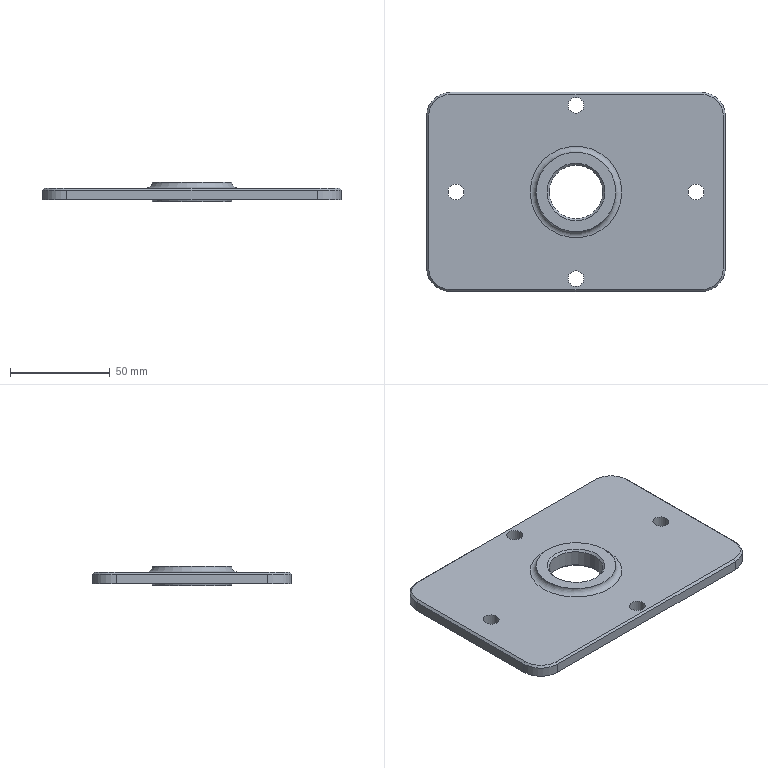Part | NX | features DATUM_CSYS 2, BLEND 1, BREP 1, CHAMFER 1, CPROJ 1, EXTRUDE 1, SKETCH 1 | 1 solid | 38 faces | box 150 x 100 x 10 mm | volume 75362 mm3 | plane 13 | cylinder 13 | cone 6 | torus 6 | commonest cylinder face diameters 4 x4 8 x4 24 x4 27 x1
STEP:
#1=CARTESIAN_POINT('',(15.75,378.,376.084));
#2=VERTEX_POINT('',#1);
#3=CARTESIAN_POINT('',(19.75,378.,376.084));
#4=DIRECTION('',(0.,0.,-1.));
#5=DIRECTION('',(-1.,0.,0.));
#6=AXIS2_PLACEMENT_3D('',#3,#4,#5);
#7=CIRCLE('',#6,4.);
#8=EDGE_CURVE('',#2,#2,#7,.T.);
#9=ORIENTED_EDGE('',*,*,#8,.F.);
#10=EDGE_LOOP('',(#9));
#11=FACE_BOUND('',#10,.T.);
#12=CARTESIAN_POINT('',(136.25,378.,376.084));
#13=VERTEX_POINT('',#12);
#14=CARTESIAN_POINT('',(140.25,378.,376.084));
#15=DIRECTION('',(0.,0.,-1.));
#16=DIRECTION('',(-1.,0.,0.));
#17=AXIS2_PLACEMENT_3D('',#14,#15,#16);
#18=CIRCLE('',#17,4.);
#19=EDGE_CURVE('',#13,#13,#18,.T.);
#20=ORIENTED_EDGE('',*,*,#19,.F.);
#21=EDGE_LOOP('',(#20));
#22=FACE_BOUND('',#21,.T.);
#23=CARTESIAN_POINT('',(126.,340.5,376.084));
#24=VERTEX_POINT('',#23);
#25=CARTESIAN_POINT('',(130.,344.5,376.084));
#26=VERTEX_POINT('',#25);
#27=CARTESIAN_POINT('',(126.,344.5,376.084));
#28=DIRECTION('',(0.,0.,1.));
#29=DIRECTION('',(1.,0.,0.));
#30=AXIS2_PLACEMENT_3D('',#27,#28,#29);
#31=CIRCLE('',#30,4.);
#32=EDGE_CURVE('',#24,#26,#31,.T.);
#33=ORIENTED_EDGE('',*,*,#32,.T.);
#34=CARTESIAN_POINT('',(130.,411.5,376.084));
#35=VERTEX_POINT('',#34);
#36=CARTESIAN_POINT('',(130.,344.5,376.084));
#37=DIRECTION('',(0.,-1.,0.));
#38=VECTOR('',#37,1000.);
#39=LINE('',#36,#38);
#40=EDGE_CURVE('',#26,#35,#39,.F.);
#41=ORIENTED_EDGE('',*,*,#40,.T.);
#42=CARTESIAN_POINT('',(126.,415.5,376.084));
#43=VERTEX_POINT('',#42);
#44=CARTESIAN_POINT('',(126.,411.5,376.084));
#45=DIRECTION('',(0.,0.,1.));
#46=DIRECTION('',(1.,0.,0.));
#47=AXIS2_PLACEMENT_3D('',#44,#45,#46);
#48=CIRCLE('',#47,4.);
#49=EDGE_CURVE('',#35,#43,#48,.T.);
#50=ORIENTED_EDGE('',*,*,#49,.T.);
#51=CARTESIAN_POINT('',(34.,415.5,376.084));
#52=VERTEX_POINT('',#51);
#53=CARTESIAN_POINT('',(126.,415.5,376.084));
#54=DIRECTION('',(1.,0.,0.));
#55=VECTOR('',#54,1000.);
#56=LINE('',#53,#55);
#57=EDGE_CURVE('',#43,#52,#56,.F.);
#58=ORIENTED_EDGE('',*,*,#57,.T.);
#59=CARTESIAN_POINT('',(30.,411.5,376.084));
#60=VERTEX_POINT('',#59);
#61=CARTESIAN_POINT('',(34.,411.5,376.084));
#62=DIRECTION('',(0.,0.,1.));
#63=DIRECTION('',(1.,0.,0.));
#64=AXIS2_PLACEMENT_3D('',#61,#62,#63);
#65=CIRCLE('',#64,4.);
#66=EDGE_CURVE('',#52,#60,#65,.T.);
#67=ORIENTED_EDGE('',*,*,#66,.T.);
#68=CARTESIAN_POINT('',(30.,344.5,376.084));
#69=VERTEX_POINT('',#68);
#70=CARTESIAN_POINT('',(30.,411.5,376.084));
#71=DIRECTION('',(0.,1.,0.));
#72=VECTOR('',#71,1000.);
#73=LINE('',#70,#72);
#74=EDGE_CURVE('',#60,#69,#73,.F.);
#75=ORIENTED_EDGE('',*,*,#74,.T.);
#76=CARTESIAN_POINT('',(34.,340.5,376.084));
#77=VERTEX_POINT('',#76);
#78=CARTESIAN_POINT('',(34.,344.5,376.084));
#79=DIRECTION('',(0.,0.,1.));
#80=DIRECTION('',(1.,0.,0.));
#81=AXIS2_PLACEMENT_3D('',#78,#79,#80);
#82=CIRCLE('',#81,4.);
#83=EDGE_CURVE('',#69,#77,#82,.T.);
#84=ORIENTED_EDGE('',*,*,#83,.T.);
#85=CARTESIAN_POINT('',(34.,340.5,376.084));
#86=DIRECTION('',(-1.,0.,0.));
#87=VECTOR('',#86,1000.);
#88=LINE('',#85,#87);
#89=EDGE_CURVE('',#77,#24,#88,.F.);
#90=ORIENTED_EDGE('',*,*,#89,.T.);
#91=EDGE_LOOP('',(#33,#41,#50,#58,#67,#75,#84,#90));
#92=FACE_BOUND('',#91,.T.);
#93=CARTESIAN_POINT('',(155.,416.,376.084));
#94=VERTEX_POINT('',#93);
#95=CARTESIAN_POINT('',(155.,340.,376.084));
#96=VERTEX_POINT('',#95);
#97=CARTESIAN_POINT('',(155.,516.,376.084));
#98=DIRECTION('',(0.,1.,0.));
#99=VECTOR('',#98,1000.);
#100=LINE('',#97,#99);
#101=EDGE_CURVE('',#94,#96,#100,.F.);
#102=ORIENTED_EDGE('',*,*,#101,.T.);
#103=CARTESIAN_POINT('',(143.,328.,376.084));
#104=VERTEX_POINT('',#103);
#105=CARTESIAN_POINT('',(143.,340.,376.084));
#106=DIRECTION('',(0.,0.,1.));
#107=DIRECTION('',(1.,0.,0.));
#108=AXIS2_PLACEMENT_3D('',#105,#106,#107);
#109=CIRCLE('',#108,12.);
#110=EDGE_CURVE('',#96,#104,#109,.F.);
#111=ORIENTED_EDGE('',*,*,#110,.T.);
#112=CARTESIAN_POINT('',(17.,328.,376.084));
#113=VERTEX_POINT('',#112);
#114=CARTESIAN_POINT('',(160.,328.,376.084));
#115=DIRECTION('',(1.,0.,0.));
#116=VECTOR('',#115,1000.);
#117=LINE('',#114,#116);
#118=EDGE_CURVE('',#104,#113,#117,.F.);
#119=ORIENTED_EDGE('',*,*,#118,.T.);
#120=CARTESIAN_POINT('',(5.,340.,376.084));
#121=VERTEX_POINT('',#120);
#122=CARTESIAN_POINT('',(17.,340.,376.084));
#123=DIRECTION('',(0.,0.,1.));
#124=DIRECTION('',(1.,0.,0.));
#125=AXIS2_PLACEMENT_3D('',#122,#123,#124);
#126=CIRCLE('',#125,12.);
#127=EDGE_CURVE('',#113,#121,#126,.F.);
#128=ORIENTED_EDGE('',*,*,#127,.T.);
#129=CARTESIAN_POINT('',(5.,416.,376.084));
#130=VERTEX_POINT('',#129);
#131=CARTESIAN_POINT('',(5.,516.,376.084));
#132=DIRECTION('',(0.,-1.,0.));
#133=VECTOR('',#132,1000.);
#134=LINE('',#131,#133);
#135=EDGE_CURVE('',#121,#130,#134,.F.);
#136=ORIENTED_EDGE('',*,*,#135,.T.);
#137=CARTESIAN_POINT('',(17.,428.,376.084));
#138=VERTEX_POINT('',#137);
#139=CARTESIAN_POINT('',(17.,416.,376.084));
#140=DIRECTION('',(0.,0.,1.));
#141=DIRECTION('',(1.,0.,0.));
#142=AXIS2_PLACEMENT_3D('',#139,#140,#141);
#143=CIRCLE('',#142,12.);
#144=EDGE_CURVE('',#138,#130,#143,.T.);
#145=ORIENTED_EDGE('',*,*,#144,.F.);
#146=CARTESIAN_POINT('',(143.,428.,376.084));
#147=VERTEX_POINT('',#146);
#148=CARTESIAN_POINT('',(160.,428.,376.084));
#149=DIRECTION('',(-1.,0.,0.));
#150=VECTOR('',#149,1000.);
#151=LINE('',#148,#150);
#152=EDGE_CURVE('',#138,#147,#151,.F.);
#153=ORIENTED_EDGE('',*,*,#152,.T.);
#154=CARTESIAN_POINT('',(143.,416.,376.084));
#155=DIRECTION('',(0.,0.,1.));
#156=DIRECTION('',(1.,0.,0.));
#157=AXIS2_PLACEMENT_3D('',#154,#155,#156);
#158=CIRCLE('',#157,12.);
#159=EDGE_CURVE('',#147,#94,#158,.F.);
#160=ORIENTED_EDGE('',*,*,#159,.T.);
#161=EDGE_LOOP('',(#102,#111,#119,#128,#136,#145,#153,#160));
#162=FACE_BOUND('',#161,.T.);
#163=CARTESIAN_POINT('',(76.,334.5,376.084));
#164=VERTEX_POINT('',#163);
#165=CARTESIAN_POINT('',(80.,334.5,376.084));
#166=DIRECTION('',(0.,0.,-1.));
#167=DIRECTION('',(-1.,0.,0.));
#168=AXIS2_PLACEMENT_3D('',#165,#166,#167);
#169=CIRCLE('',#168,4.);
#170=EDGE_CURVE('',#164,#164,#169,.T.);
#171=ORIENTED_EDGE('',*,*,#170,.F.);
#172=EDGE_LOOP('',(#171));
#173=FACE_BOUND('',#172,.T.);
#174=CARTESIAN_POINT('',(76.,421.5,376.084));
#175=VERTEX_POINT('',#174);
#176=CARTESIAN_POINT('',(80.,421.5,376.084));
#177=DIRECTION('',(0.,0.,-1.));
#178=DIRECTION('',(-1.,0.,0.));
#179=AXIS2_PLACEMENT_3D('',#176,#177,#178);
#180=CIRCLE('',#179,4.);
#181=EDGE_CURVE('',#175,#175,#180,.F.);
#182=ORIENTED_EDGE('',*,*,#181,.T.);
#183=EDGE_LOOP('',(#182));
#184=FACE_BOUND('',#183,.T.);
#185=CARTESIAN_POINT('',(80.,378.,376.084));
#186=DIRECTION('',(0.,0.,-1.));
#187=DIRECTION('',(-1.,0.,0.));
#188=AXIS2_PLACEMENT_3D('',#185,#186,#187);
#189=PLANE('',#188);
#190=ADVANCED_FACE('',(#11,#22,#92,#162,#173,#184),#189,.T.);
#191=CARTESIAN_POINT('',(76.,334.5,382.084));
#192=VERTEX_POINT('',#191);
#193=CARTESIAN_POINT('',(80.,334.5,382.084));
#194=DIRECTION('',(0.,0.,-1.));
#195=DIRECTION('',(-1.,0.,0.));
#196=AXIS2_PLACEMENT_3D('',#193,#194,#195);
#197=CIRCLE('',#196,4.);
#198=EDGE_CURVE('',#192,#192,#197,.F.);
#199=ORIENTED_EDGE('',*,*,#198,.T.);
#200=EDGE_LOOP('',(#199));
#201=FACE_BOUND('',#200,.T.);
#202=ORIENTED_EDGE('',*,*,#170,.T.);
#203=EDGE_LOOP('',(#202));
#204=FACE_BOUND('',#203,.T.);
#205=CARTESIAN_POINT('',(80.,334.5,402.084));
#206=DIRECTION('',(0.,0.,-1.));
#207=DIRECTION('',(-1.,0.,0.));
#208=AXIS2_PLACEMENT_3D('',#205,#206,#207);
#209=CYLINDRICAL_SURFACE('',#208,4.);
#210=ADVANCED_FACE('',(#201,#204),#209,.F.);
#211=CARTESIAN_POINT('',(76.,421.5,382.084));
#212=VERTEX_POINT('',#211);
#213=CARTESIAN_POINT('',(80.,421.5,382.084));
#214=DIRECTION('',(0.,0.,-1.));
#215=DIRECTION('',(-1.,0.,0.));
#216=AXIS2_PLACEMENT_3D('',#213,#214,#215);
#217=CIRCLE('',#216,4.);
#218=EDGE_CURVE('',#212,#212,#217,.T.);
#219=ORIENTED_EDGE('',*,*,#218,.F.);
#220=EDGE_LOOP('',(#219));
#221=FACE_BOUND('',#220,.T.);
#222=ORIENTED_EDGE('',*,*,#181,.F.);
#223=EDGE_LOOP('',(#222));
#224=FACE_BOUND('',#223,.T.);
#225=CARTESIAN_POINT('',(80.,421.5,402.084));
#226=DIRECTION('',(0.,0.,-1.));
#227=DIRECTION('',(-1.,0.,0.));
#228=AXIS2_PLACEMENT_3D('',#225,#226,#227);
#229=CYLINDRICAL_SURFACE('',#228,4.);
#230=ADVANCED_FACE('',(#221,#224),#229,.F.);
#231=CARTESIAN_POINT('',(15.75,378.,382.084));
#232=VERTEX_POINT('',#231);
#233=CARTESIAN_POINT('',(19.75,378.,382.084));
#234=DIRECTION('',(0.,0.,-1.));
#235=DIRECTION('',(-1.,0.,0.));
#236=AXIS2_PLACEMENT_3D('',#233,#234,#235);
#237=CIRCLE('',#236,4.);
#238=EDGE_CURVE('',#232,#232,#237,.T.);
#239=ORIENTED_EDGE('',*,*,#238,.F.);
#240=EDGE_LOOP('',(#239));
#241=FACE_BOUND('',#240,.T.);
#242=ORIENTED_EDGE('',*,*,#8,.T.);
#243=EDGE_LOOP('',(#242));
#244=FACE_BOUND('',#243,.T.);
#245=CARTESIAN_POINT('',(19.75,378.,402.084));
#246=DIRECTION('',(0.,0.,-1.));
#247=DIRECTION('',(-1.,0.,0.));
#248=AXIS2_PLACEMENT_3D('',#245,#246,#247);
#249=CYLINDRICAL_SURFACE('',#248,4.);
#250=ADVANCED_FACE('',(#241,#244),#249,.F.);
#251=CARTESIAN_POINT('',(154.,340.,382.084));
#252=VERTEX_POINT('',#251);
#253=CARTESIAN_POINT('',(155.,340.,381.084));
#254=VERTEX_POINT('',#253);
#255=CARTESIAN_POINT('',(154.,340.,382.084));
#256=DIRECTION('',(0.7071,0.,-0.7071));
#257=VECTOR('',#256,1000.);
#258=LINE('',#255,#257);
#259=EDGE_CURVE('',#252,#254,#258,.T.);
#260=ORIENTED_EDGE('',*,*,#259,.F.);
#261=CARTESIAN_POINT('',(143.,329.,382.084));
#262=VERTEX_POINT('',#261);
#263=CARTESIAN_POINT('',(143.,340.,382.084));
#264=DIRECTION('',(0.,0.,-1.));
#265=DIRECTION('',(-1.,0.,0.));
#266=AXIS2_PLACEMENT_3D('',#263,#264,#265);
#267=CIRCLE('',#266,11.);
#268=EDGE_CURVE('',#262,#252,#267,.F.);
#269=ORIENTED_EDGE('',*,*,#268,.F.);
#270=CARTESIAN_POINT('',(143.,328.,381.084));
#271=VERTEX_POINT('',#270);
#272=CARTESIAN_POINT('',(143.,328.,381.084));
#273=DIRECTION('',(0.,0.7071,0.7071));
#274=VECTOR('',#273,1000.);
#275=LINE('',#272,#274);
#276=EDGE_CURVE('',#271,#262,#275,.T.);
#277=ORIENTED_EDGE('',*,*,#276,.F.);
#278=CARTESIAN_POINT('',(143.,340.,381.084));
#279=DIRECTION('',(0.,0.,-1.));
#280=DIRECTION('',(-1.,0.,0.));
#281=AXIS2_PLACEMENT_3D('',#278,#279,#280);
#282=CIRCLE('',#281,12.);
#283=EDGE_CURVE('',#254,#271,#282,.T.);
#284=ORIENTED_EDGE('',*,*,#283,.F.);
#285=EDGE_LOOP('',(#260,#269,#277,#284));
#286=FACE_BOUND('',#285,.T.);
#287=CARTESIAN_POINT('',(143.,340.,381.084));
#288=DIRECTION('',(0.,0.,-1.));
#289=DIRECTION('',(-1.,0.,0.));
#290=AXIS2_PLACEMENT_3D('',#287,#288,#289);
#291=CONICAL_SURFACE('',#290,12.,0.7854);
#292=ADVANCED_FACE('',(#286),#291,.T.);
#293=ORIENTED_EDGE('',*,*,#276,.T.);
#294=CARTESIAN_POINT('',(17.,329.,382.084));
#295=VERTEX_POINT('',#294);
#296=CARTESIAN_POINT('',(143.,329.,382.084));
#297=DIRECTION('',(1.,0.,0.));
#298=VECTOR('',#297,1000.);
#299=LINE('',#296,#298);
#300=EDGE_CURVE('',#295,#262,#299,.T.);
#301=ORIENTED_EDGE('',*,*,#300,.F.);
#302=CARTESIAN_POINT('',(17.,328.,381.084));
#303=VERTEX_POINT('',#302);
#304=CARTESIAN_POINT('',(17.,328.,381.084));
#305=DIRECTION('',(0.,0.7071,0.7071));
#306=VECTOR('',#305,1000.);
#307=LINE('',#304,#306);
#308=EDGE_CURVE('',#303,#295,#307,.T.);
#309=ORIENTED_EDGE('',*,*,#308,.F.);
#310=CARTESIAN_POINT('',(17.,328.,381.084));
#311=DIRECTION('',(-1.,0.,0.));
#312=VECTOR('',#311,1000.);
#313=LINE('',#310,#312);
#314=EDGE_CURVE('',#271,#303,#313,.T.);
#315=ORIENTED_EDGE('',*,*,#314,.F.);
#316=EDGE_LOOP('',(#293,#301,#309,#315));
#317=FACE_BOUND('',#316,.T.);
#318=CARTESIAN_POINT('',(143.,328.,381.084));
#319=DIRECTION('',(0.,-0.7071,0.7071));
#320=DIRECTION('',(1.,0.,0.));
#321=AXIS2_PLACEMENT_3D('',#318,#319,#320);
#322=PLANE('',#321);
#323=ADVANCED_FACE('',(#317),#322,.T.);
#324=ORIENTED_EDGE('',*,*,#259,.T.);
#325=CARTESIAN_POINT('',(155.,416.,381.084));
#326=VERTEX_POINT('',#325);
#327=CARTESIAN_POINT('',(155.,340.,381.084));
#328=DIRECTION('',(0.,-1.,0.));
#329=VECTOR('',#328,1000.);
#330=LINE('',#327,#329);
#331=EDGE_CURVE('',#326,#254,#330,.T.);
#332=ORIENTED_EDGE('',*,*,#331,.F.);
#333=CARTESIAN_POINT('',(154.,416.,382.084));
#334=VERTEX_POINT('',#333);
#335=CARTESIAN_POINT('',(154.,416.,382.084));
#336=DIRECTION('',(0.7071,0.,-0.7071));
#337=VECTOR('',#336,1000.);
#338=LINE('',#335,#337);
#339=EDGE_CURVE('',#334,#326,#338,.T.);
#340=ORIENTED_EDGE('',*,*,#339,.F.);
#341=CARTESIAN_POINT('',(154.,416.,382.084));
#342=DIRECTION('',(0.,1.,0.));
#343=VECTOR('',#342,1000.);
#344=LINE('',#341,#343);
#345=EDGE_CURVE('',#252,#334,#344,.T.);
#346=ORIENTED_EDGE('',*,*,#345,.F.);
#347=EDGE_LOOP('',(#324,#332,#340,#346));
#348=FACE_BOUND('',#347,.T.);
#349=CARTESIAN_POINT('',(155.,416.,381.084));
#350=DIRECTION('',(0.7071,0.,0.7071));
#351=DIRECTION('',(0.,1.,0.));
#352=AXIS2_PLACEMENT_3D('',#349,#350,#351);
#353=PLANE('',#352);
#354=ADVANCED_FACE('',(#348),#353,.T.);
#355=ORIENTED_EDGE('',*,*,#308,.T.);
#356=CARTESIAN_POINT('',(6.,340.,382.084));
#357=VERTEX_POINT('',#356);
#358=CARTESIAN_POINT('',(17.,340.,382.084));
#359=DIRECTION('',(0.,0.,-1.));
#360=DIRECTION('',(-1.,0.,0.));
#361=AXIS2_PLACEMENT_3D('',#358,#359,#360);
#362=CIRCLE('',#361,11.);
#363=EDGE_CURVE('',#357,#295,#362,.F.);
#364=ORIENTED_EDGE('',*,*,#363,.F.);
#365=CARTESIAN_POINT('',(5.,340.,381.084));
#366=VERTEX_POINT('',#365);
#367=CARTESIAN_POINT('',(5.,340.,381.084));
#368=DIRECTION('',(0.7071,0.,0.7071));
#369=VECTOR('',#368,1000.);
#370=LINE('',#367,#369);
#371=EDGE_CURVE('',#366,#357,#370,.T.);
#372=ORIENTED_EDGE('',*,*,#371,.F.);
#373=CARTESIAN_POINT('',(17.,340.,381.084));
#374=DIRECTION('',(0.,0.,-1.));
#375=DIRECTION('',(-1.,0.,0.));
#376=AXIS2_PLACEMENT_3D('',#373,#374,#375);
#377=CIRCLE('',#376,12.);
#378=EDGE_CURVE('',#303,#366,#377,.T.);
#379=ORIENTED_EDGE('',*,*,#378,.F.);
#380=EDGE_LOOP('',(#355,#364,#372,#379));
#381=FACE_BOUND('',#380,.T.);
#382=CARTESIAN_POINT('',(17.,340.,381.084));
#383=DIRECTION('',(0.,0.,-1.));
#384=DIRECTION('',(-1.,0.,0.));
#385=AXIS2_PLACEMENT_3D('',#382,#383,#384);
#386=CONICAL_SURFACE('',#385,12.,0.7854);
#387=ADVANCED_FACE('',(#381),#386,.T.);
#388=ORIENTED_EDGE('',*,*,#339,.T.);
#389=CARTESIAN_POINT('',(143.,428.,381.084));
#390=VERTEX_POINT('',#389);
#391=CARTESIAN_POINT('',(143.,416.,381.084));
#392=DIRECTION('',(0.,0.,-1.));
#393=DIRECTION('',(-1.,0.,0.));
#394=AXIS2_PLACEMENT_3D('',#391,#392,#393);
#395=CIRCLE('',#394,12.);
#396=EDGE_CURVE('',#390,#326,#395,.T.);
#397=ORIENTED_EDGE('',*,*,#396,.F.);
#398=CARTESIAN_POINT('',(143.,427.,382.084));
#399=VERTEX_POINT('',#398);
#400=CARTESIAN_POINT('',(143.,427.,382.084));
#401=DIRECTION('',(0.,0.7071,-0.7071));
#402=VECTOR('',#401,1000.);
#403=LINE('',#400,#402);
#404=EDGE_CURVE('',#399,#390,#403,.T.);
#405=ORIENTED_EDGE('',*,*,#404,.F.);
#406=CARTESIAN_POINT('',(143.,416.,382.084));
#407=DIRECTION('',(0.,0.,-1.));
#408=DIRECTION('',(-1.,0.,0.));
#409=AXIS2_PLACEMENT_3D('',#406,#407,#408);
#410=CIRCLE('',#409,11.);
#411=EDGE_CURVE('',#334,#399,#410,.F.);
#412=ORIENTED_EDGE('',*,*,#411,.F.);
#413=EDGE_LOOP('',(#388,#397,#405,#412));
#414=FACE_BOUND('',#413,.T.);
#415=CARTESIAN_POINT('',(143.,416.,381.084));
#416=DIRECTION('',(0.,0.,-1.));
#417=DIRECTION('',(-1.,0.,0.));
#418=AXIS2_PLACEMENT_3D('',#415,#416,#417);
#419=CONICAL_SURFACE('',#418,12.,0.7854);
#420=ADVANCED_FACE('',(#414),#419,.T.);
#421=ORIENTED_EDGE('',*,*,#371,.T.);
#422=CARTESIAN_POINT('',(6.,416.,382.084));
#423=VERTEX_POINT('',#422);
#424=CARTESIAN_POINT('',(6.,340.,382.084));
#425=DIRECTION('',(0.,-1.,0.));
#426=VECTOR('',#425,1000.);
#427=LINE('',#424,#426);
#428=EDGE_CURVE('',#423,#357,#427,.T.);
#429=ORIENTED_EDGE('',*,*,#428,.F.);
#430=CARTESIAN_POINT('',(5.,416.,381.084));
#431=VERTEX_POINT('',#430);
#432=CARTESIAN_POINT('',(5.,416.,381.084));
#433=DIRECTION('',(0.7071,0.,0.7071));
#434=VECTOR('',#433,1000.);
#435=LINE('',#432,#434);
#436=EDGE_CURVE('',#431,#423,#435,.T.);
#437=ORIENTED_EDGE('',*,*,#436,.F.);
#438=CARTESIAN_POINT('',(5.,416.,381.084));
#439=DIRECTION('',(0.,1.,0.));
#440=VECTOR('',#439,1000.);
#441=LINE('',#438,#440);
#442=EDGE_CURVE('',#366,#431,#441,.T.);
#443=ORIENTED_EDGE('',*,*,#442,.F.);
#444=EDGE_LOOP('',(#421,#429,#437,#443));
#445=FACE_BOUND('',#444,.T.);
#446=CARTESIAN_POINT('',(5.,340.,381.084));
#447=DIRECTION('',(-0.7071,0.,0.7071));
#448=DIRECTION('',(0.,-1.,0.));
#449=AXIS2_PLACEMENT_3D('',#446,#447,#448);
#450=PLANE('',#449);
#451=ADVANCED_FACE('',(#445),#450,.T.);
#452=ORIENTED_EDGE('',*,*,#404,.T.);
#453=CARTESIAN_POINT('',(17.,428.,381.084));
#454=VERTEX_POINT('',#453);
#455=CARTESIAN_POINT('',(143.,428.,381.084));
#456=DIRECTION('',(1.,0.,0.));
#457=VECTOR('',#456,1000.);
#458=LINE('',#455,#457);
#459=EDGE_CURVE('',#454,#390,#458,.T.);
#460=ORIENTED_EDGE('',*,*,#459,.F.);
#461=CARTESIAN_POINT('',(17.,427.,382.084));
#462=VERTEX_POINT('',#461);
#463=CARTESIAN_POINT('',(17.,427.,382.084));
#464=DIRECTION('',(0.,0.7071,-0.7071));
#465=VECTOR('',#464,1000.);
#466=LINE('',#463,#465);
#467=EDGE_CURVE('',#462,#454,#466,.T.);
#468=ORIENTED_EDGE('',*,*,#467,.F.);
#469=CARTESIAN_POINT('',(17.,427.,382.084));
#470=DIRECTION('',(-1.,0.,0.));
#471=VECTOR('',#470,1000.);
#472=LINE('',#469,#471);
#473=EDGE_CURVE('',#399,#462,#472,.T.);
#474=ORIENTED_EDGE('',*,*,#473,.F.);
#475=EDGE_LOOP('',(#452,#460,#468,#474));
#476=FACE_BOUND('',#475,.T.);
#477=CARTESIAN_POINT('',(17.,428.,381.084));
#478=DIRECTION('',(0.,0.7071,0.7071));
#479=DIRECTION('',(-1.,0.,0.));
#480=AXIS2_PLACEMENT_3D('',#477,#478,#479);
#481=PLANE('',#480);
#482=ADVANCED_FACE('',(#476),#481,.T.);
#483=ORIENTED_EDGE('',*,*,#436,.T.);
#484=CARTESIAN_POINT('',(17.,416.,382.084));
#485=DIRECTION('',(0.,0.,-1.));
#486=DIRECTION('',(-1.,0.,0.));
#487=AXIS2_PLACEMENT_3D('',#484,#485,#486);
#488=CIRCLE('',#487,11.);
#489=EDGE_CURVE('',#462,#423,#488,.F.);
#490=ORIENTED_EDGE('',*,*,#489,.F.);
#491=ORIENTED_EDGE('',*,*,#467,.T.);
#492=CARTESIAN_POINT('',(17.,416.,381.084));
#493=DIRECTION('',(0.,0.,-1.));
#494=DIRECTION('',(-1.,0.,0.));
#495=AXIS2_PLACEMENT_3D('',#492,#493,#494);
#496=CIRCLE('',#495,12.);
#497=EDGE_CURVE('',#431,#454,#496,.T.);
#498=ORIENTED_EDGE('',*,*,#497,.F.);
#499=EDGE_LOOP('',(#483,#490,#491,#498));
#500=FACE_BOUND('',#499,.T.);
#501=CARTESIAN_POINT('',(17.,416.,381.084));
#502=DIRECTION('',(0.,0.,-1.));
#503=DIRECTION('',(-1.,0.,0.));
#504=AXIS2_PLACEMENT_3D('',#501,#502,#503);
#505=CONICAL_SURFACE('',#504,12.,0.7854);
#506=ADVANCED_FACE('',(#500),#505,.T.);
#507=CARTESIAN_POINT('',(5.,416.,382.084));
#508=DIRECTION('',(0.,0.,-1.));
#509=VECTOR('',#508,1000.);
#510=LINE('',#507,#509);
#511=EDGE_CURVE('',#431,#130,#510,.T.);
#512=ORIENTED_EDGE('',*,*,#511,.F.);
#513=ORIENTED_EDGE('',*,*,#497,.T.);
#514=CARTESIAN_POINT('',(17.,428.,382.084));
#515=DIRECTION('',(0.,0.,-1.));
#516=VECTOR('',#515,1000.);
#517=LINE('',#514,#516);
#518=EDGE_CURVE('',#454,#138,#517,.T.);
#519=ORIENTED_EDGE('',*,*,#518,.T.);
#520=ORIENTED_EDGE('',*,*,#144,.T.);
#521=EDGE_LOOP('',(#512,#513,#519,#520));
#522=FACE_BOUND('',#521,.T.);
#523=CARTESIAN_POINT('',(17.,416.,382.084));
#524=DIRECTION('',(0.,0.,-1.));
#525=DIRECTION('',(-1.,0.,0.));
#526=AXIS2_PLACEMENT_3D('',#523,#524,#525);
#527=CYLINDRICAL_SURFACE('',#526,12.);
#528=ADVANCED_FACE('',(#522),#527,.T.);
#529=ORIENTED_EDGE('',*,*,#518,.F.);
#530=ORIENTED_EDGE('',*,*,#459,.T.);
#531=CARTESIAN_POINT('',(143.,428.,382.084));
#532=DIRECTION('',(0.,0.,-1.));
#533=VECTOR('',#532,1000.);
#534=LINE('',#531,#533);
#535=EDGE_CURVE('',#390,#147,#534,.T.);
#536=ORIENTED_EDGE('',*,*,#535,.T.);
#537=ORIENTED_EDGE('',*,*,#152,.F.);
#538=EDGE_LOOP('',(#529,#530,#536,#537));
#539=FACE_BOUND('',#538,.T.);
#540=CARTESIAN_POINT('',(17.,428.,382.084));
#541=DIRECTION('',(0.,1.,0.));
#542=DIRECTION('',(-1.,0.,0.));
#543=AXIS2_PLACEMENT_3D('',#540,#541,#542);
#544=PLANE('',#543);
#545=ADVANCED_FACE('',(#539),#544,.T.);
#546=CARTESIAN_POINT('',(5.,340.,382.084));
#547=DIRECTION('',(0.,0.,-1.));
#548=VECTOR('',#547,1000.);
#549=LINE('',#546,#548);
#550=EDGE_CURVE('',#366,#121,#549,.T.);
#551=ORIENTED_EDGE('',*,*,#550,.F.);
#552=ORIENTED_EDGE('',*,*,#442,.T.);
#553=ORIENTED_EDGE('',*,*,#511,.T.);
#554=ORIENTED_EDGE('',*,*,#135,.F.);
#555=EDGE_LOOP('',(#551,#552,#553,#554));
#556=FACE_BOUND('',#555,.T.);
#557=CARTESIAN_POINT('',(5.,340.,382.084));
#558=DIRECTION('',(-1.,0.,0.));
#559=DIRECTION('',(0.,0.,1.));
#560=AXIS2_PLACEMENT_3D('',#557,#558,#559);
#561=PLANE('',#560);
#562=ADVANCED_FACE('',(#556),#561,.T.);
#563=ORIENTED_EDGE('',*,*,#535,.F.);
#564=ORIENTED_EDGE('',*,*,#396,.T.);
#565=CARTESIAN_POINT('',(155.,416.,382.084));
#566=DIRECTION('',(0.,0.,-1.));
#567=VECTOR('',#566,1000.);
#568=LINE('',#565,#567);
#569=EDGE_CURVE('',#326,#94,#568,.T.);
#570=ORIENTED_EDGE('',*,*,#569,.T.);
#571=ORIENTED_EDGE('',*,*,#159,.F.);
#572=EDGE_LOOP('',(#563,#564,#570,#571));
#573=FACE_BOUND('',#572,.T.);
#574=CARTESIAN_POINT('',(143.,416.,382.084));
#575=DIRECTION('',(0.,0.,-1.));
#576=DIRECTION('',(-1.,0.,0.));
#577=AXIS2_PLACEMENT_3D('',#574,#575,#576);
#578=CYLINDRICAL_SURFACE('',#577,12.);
#579=ADVANCED_FACE('',(#573),#578,.T.);
#580=CARTESIAN_POINT('',(17.,328.,382.084));
#581=DIRECTION('',(0.,0.,-1.));
#582=VECTOR('',#581,1000.);
#583=LINE('',#580,#582);
#584=EDGE_CURVE('',#303,#113,#583,.T.);
#585=ORIENTED_EDGE('',*,*,#584,.F.);
#586=ORIENTED_EDGE('',*,*,#378,.T.);
#587=ORIENTED_EDGE('',*,*,#550,.T.);
#588=ORIENTED_EDGE('',*,*,#127,.F.);
#589=EDGE_LOOP('',(#585,#586,#587,#588));
#590=FACE_BOUND('',#589,.T.);
#591=CARTESIAN_POINT('',(17.,340.,382.084));
#592=DIRECTION('',(0.,0.,-1.));
#593=DIRECTION('',(-1.,0.,0.));
#594=AXIS2_PLACEMENT_3D('',#591,#592,#593);
#595=CYLINDRICAL_SURFACE('',#594,12.);
#596=ADVANCED_FACE('',(#590),#595,.T.);
#597=ORIENTED_EDGE('',*,*,#569,.F.);
#598=ORIENTED_EDGE('',*,*,#331,.T.);
#599=CARTESIAN_POINT('',(155.,340.,382.084));
#600=DIRECTION('',(0.,0.,-1.));
#601=VECTOR('',#600,1000.);
#602=LINE('',#599,#601);
#603=EDGE_CURVE('',#254,#96,#602,.T.);
#604=ORIENTED_EDGE('',*,*,#603,.T.);
#605=ORIENTED_EDGE('',*,*,#101,.F.);
#606=EDGE_LOOP('',(#597,#598,#604,#605));
#607=FACE_BOUND('',#606,.T.);
#608=CARTESIAN_POINT('',(155.,416.,382.084));
#609=DIRECTION('',(1.,0.,0.));
#610=DIRECTION('',(0.,0.,-1.));
#611=AXIS2_PLACEMENT_3D('',#608,#609,#610);
#612=PLANE('',#611);
#613=ADVANCED_FACE('',(#607),#612,.T.);
#614=CARTESIAN_POINT('',(143.,328.,382.084));
#615=DIRECTION('',(0.,0.,-1.));
#616=VECTOR('',#615,1000.);
#617=LINE('',#614,#616);
#618=EDGE_CURVE('',#271,#104,#617,.T.);
#619=ORIENTED_EDGE('',*,*,#618,.F.);
#620=ORIENTED_EDGE('',*,*,#314,.T.);
#621=ORIENTED_EDGE('',*,*,#584,.T.);
#622=ORIENTED_EDGE('',*,*,#118,.F.);
#623=EDGE_LOOP('',(#619,#620,#621,#622));
#624=FACE_BOUND('',#623,.T.);
#625=CARTESIAN_POINT('',(143.,328.,382.084));
#626=DIRECTION('',(0.,-1.,0.));
#627=DIRECTION('',(1.,0.,0.));
#628=AXIS2_PLACEMENT_3D('',#625,#626,#627);
#629=PLANE('',#628);
#630=ADVANCED_FACE('',(#624),#629,.T.);
#631=ORIENTED_EDGE('',*,*,#603,.F.);
#632=ORIENTED_EDGE('',*,*,#283,.T.);
#633=ORIENTED_EDGE('',*,*,#618,.T.);
#634=ORIENTED_EDGE('',*,*,#110,.F.);
#635=EDGE_LOOP('',(#631,#632,#633,#634));
#636=FACE_BOUND('',#635,.T.);
#637=CARTESIAN_POINT('',(143.,340.,382.084));
#638=DIRECTION('',(0.,0.,-1.));
#639=DIRECTION('',(-1.,0.,0.));
#640=AXIS2_PLACEMENT_3D('',#637,#638,#639);
#641=CYLINDRICAL_SURFACE('',#640,12.);
#642=ADVANCED_FACE('',(#636),#641,.T.);
#643=CARTESIAN_POINT('',(57.,378.,382.084));
#644=VERTEX_POINT('',#643);
#645=CARTESIAN_POINT('',(80.,378.,382.084));
#646=DIRECTION('',(0.,0.,-1.));
#647=DIRECTION('',(-1.,0.,0.));
#648=AXIS2_PLACEMENT_3D('',#645,#646,#647);
#649=CIRCLE('',#648,23.);
#650=EDGE_CURVE('',#644,#644,#649,.T.);
#651=ORIENTED_EDGE('',*,*,#650,.T.);
#652=EDGE_LOOP('',(#651));
#653=FACE_BOUND('',#652,.T.);
#654=ORIENTED_EDGE('',*,*,#473,.T.);
#655=ORIENTED_EDGE('',*,*,#489,.T.);
#656=ORIENTED_EDGE('',*,*,#428,.T.);
#657=ORIENTED_EDGE('',*,*,#363,.T.);
#658=ORIENTED_EDGE('',*,*,#300,.T.);
#659=ORIENTED_EDGE('',*,*,#268,.T.);
#660=ORIENTED_EDGE('',*,*,#345,.T.);
#661=ORIENTED_EDGE('',*,*,#411,.T.);
#662=EDGE_LOOP('',(#654,#655,#656,#657,#658,#659,#660,#661));
#663=FACE_BOUND('',#662,.T.);
#664=ORIENTED_EDGE('',*,*,#238,.T.);
#665=EDGE_LOOP('',(#664));
#666=FACE_BOUND('',#665,.T.);
#667=ORIENTED_EDGE('',*,*,#218,.T.);
#668=EDGE_LOOP('',(#667));
#669=FACE_BOUND('',#668,.T.);
#670=ORIENTED_EDGE('',*,*,#198,.F.);
#671=EDGE_LOOP('',(#670));
#672=FACE_BOUND('',#671,.T.);
#673=CARTESIAN_POINT('',(136.25,378.,382.084));
#674=VERTEX_POINT('',#673);
#675=CARTESIAN_POINT('',(140.25,378.,382.084));
#676=DIRECTION('',(0.,0.,-1.));
#677=DIRECTION('',(-1.,0.,0.));
#678=AXIS2_PLACEMENT_3D('',#675,#676,#677);
#679=CIRCLE('',#678,4.);
#680=EDGE_CURVE('',#674,#674,#679,.F.);
#681=ORIENTED_EDGE('',*,*,#680,.F.);
#682=EDGE_LOOP('',(#681));
#683=FACE_BOUND('',#682,.T.);
#684=CARTESIAN_POINT('',(17.,340.,382.084));
#685=DIRECTION('',(0.,0.,-1.));
#686=DIRECTION('',(-1.,0.,0.));
#687=AXIS2_PLACEMENT_3D('',#684,#685,#686);
#688=PLANE('',#687);
#689=ADVANCED_FACE('',(#653,#663,#666,#669,#672,#683),#688,.F.);
#690=ORIENTED_EDGE('',*,*,#680,.T.);
#691=EDGE_LOOP('',(#690));
#692=FACE_BOUND('',#691,.T.);
#693=ORIENTED_EDGE('',*,*,#19,.T.);
#694=EDGE_LOOP('',(#693));
#695=FACE_BOUND('',#694,.T.);
#696=CARTESIAN_POINT('',(140.25,378.,402.084));
#697=DIRECTION('',(0.,0.,-1.));
#698=DIRECTION('',(-1.,0.,0.));
#699=AXIS2_PLACEMENT_3D('',#696,#697,#698);
#700=CYLINDRICAL_SURFACE('',#699,4.);
#701=ADVANCED_FACE('',(#692,#695),#700,.F.);
#702=CARTESIAN_POINT('',(103.,378.,378.084));
#703=VERTEX_POINT('',#702);
#704=CARTESIAN_POINT('',(80.,378.,378.084));
#705=DIRECTION('',(0.,0.,1.));
#706=DIRECTION('',(1.,0.,0.));
#707=AXIS2_PLACEMENT_3D('',#704,#705,#706);
#708=CIRCLE('',#707,23.);
#709=EDGE_CURVE('',#703,#703,#708,.T.);
#710=ORIENTED_EDGE('',*,*,#709,.T.);
#711=EDGE_LOOP('',(#710));
#712=FACE_BOUND('',#711,.T.);
#713=CARTESIAN_POINT('',(34.,342.5,378.084));
#714=VERTEX_POINT('',#713);
#715=CARTESIAN_POINT('',(32.,344.5,378.084));
#716=VERTEX_POINT('',#715);
#717=CARTESIAN_POINT('',(34.,344.5,378.084));
#718=DIRECTION('',(0.,0.,1.));
#719=DIRECTION('',(1.,0.,0.));
#720=AXIS2_PLACEMENT_3D('',#717,#718,#719);
#721=CIRCLE('',#720,2.);
#722=EDGE_CURVE('',#714,#716,#721,.F.);
#723=ORIENTED_EDGE('',*,*,#722,.T.);
#724=CARTESIAN_POINT('',(32.,411.5,378.084));
#725=VERTEX_POINT('',#724);
#726=CARTESIAN_POINT('',(32.,411.5,378.084));
#727=DIRECTION('',(0.,1.,0.));
#728=VECTOR('',#727,1000.);
#729=LINE('',#726,#728);
#730=EDGE_CURVE('',#716,#725,#729,.T.);
#731=ORIENTED_EDGE('',*,*,#730,.T.);
#732=CARTESIAN_POINT('',(34.,413.5,378.084));
#733=VERTEX_POINT('',#732);
#734=CARTESIAN_POINT('',(34.,411.5,378.084));
#735=DIRECTION('',(0.,0.,1.));
#736=DIRECTION('',(1.,0.,0.));
#737=AXIS2_PLACEMENT_3D('',#734,#735,#736);
#738=CIRCLE('',#737,2.);
#739=EDGE_CURVE('',#725,#733,#738,.F.);
#740=ORIENTED_EDGE('',*,*,#739,.T.);
#741=CARTESIAN_POINT('',(126.,413.5,378.084));
#742=VERTEX_POINT('',#741);
#743=CARTESIAN_POINT('',(34.,413.5,378.084));
#744=DIRECTION('',(1.,0.,0.));
#745=VECTOR('',#744,1000.);
#746=LINE('',#743,#745);
#747=EDGE_CURVE('',#733,#742,#746,.T.);
#748=ORIENTED_EDGE('',*,*,#747,.T.);
#749=CARTESIAN_POINT('',(128.,411.5,378.084));
#750=VERTEX_POINT('',#749);
#751=CARTESIAN_POINT('',(126.,411.5,378.084));
#752=DIRECTION('',(0.,0.,1.));
#753=DIRECTION('',(1.,0.,0.));
#754=AXIS2_PLACEMENT_3D('',#751,#752,#753);
#755=CIRCLE('',#754,2.);
#756=EDGE_CURVE('',#742,#750,#755,.F.);
#757=ORIENTED_EDGE('',*,*,#756,.T.);
#758=CARTESIAN_POINT('',(128.,344.5,378.084));
#759=VERTEX_POINT('',#758);
#760=CARTESIAN_POINT('',(128.,411.5,378.084));
#761=DIRECTION('',(0.,-1.,0.));
#762=VECTOR('',#761,1000.);
#763=LINE('',#760,#762);
#764=EDGE_CURVE('',#750,#759,#763,.T.);
#765=ORIENTED_EDGE('',*,*,#764,.T.);
#766=CARTESIAN_POINT('',(126.,342.5,378.084));
#767=VERTEX_POINT('',#766);
#768=CARTESIAN_POINT('',(126.,344.5,378.084));
#769=DIRECTION('',(0.,0.,1.));
#770=DIRECTION('',(1.,0.,0.));
#771=AXIS2_PLACEMENT_3D('',#768,#769,#770);
#772=CIRCLE('',#771,2.);
#773=EDGE_CURVE('',#759,#767,#772,.F.);
#774=ORIENTED_EDGE('',*,*,#773,.T.);
#775=CARTESIAN_POINT('',(34.,342.5,378.084));
#776=DIRECTION('',(-1.,0.,0.));
#777=VECTOR('',#776,1000.);
#778=LINE('',#775,#777);
#779=EDGE_CURVE('',#767,#714,#778,.T.);
#780=ORIENTED_EDGE('',*,*,#779,.T.);
#781=EDGE_LOOP('',(#723,#731,#740,#748,#757,#765,#774,#780));
#782=FACE_BOUND('',#781,.T.);
#783=CARTESIAN_POINT('',(34.,411.5,378.084));
#784=DIRECTION('',(0.,0.,1.));
#785=DIRECTION('',(1.,0.,0.));
#786=AXIS2_PLACEMENT_3D('',#783,#784,#785);
#787=PLANE('',#786);
#788=ADVANCED_FACE('',(#712,#782),#787,.F.);
#789=CARTESIAN_POINT('',(32.,344.5,376.084));
#790=DIRECTION('',(0.,-1.,0.));
#791=DIRECTION('',(1.,0.,0.));
#792=AXIS2_PLACEMENT_3D('',#789,#790,#791);
#793=CIRCLE('',#792,2.);
#794=EDGE_CURVE('',#716,#69,#793,.T.);
#795=ORIENTED_EDGE('',*,*,#794,.T.);
#796=ORIENTED_EDGE('',*,*,#74,.F.);
#797=CARTESIAN_POINT('',(32.,411.5,376.084));
#798=DIRECTION('',(0.,1.,0.));
#799=DIRECTION('',(0.,0.,1.));
#800=AXIS2_PLACEMENT_3D('',#797,#798,#799);
#801=CIRCLE('',#800,2.);
#802=EDGE_CURVE('',#60,#725,#801,.T.);
#803=ORIENTED_EDGE('',*,*,#802,.T.);
#804=ORIENTED_EDGE('',*,*,#730,.F.);
#805=EDGE_LOOP('',(#795,#796,#803,#804));
#806=FACE_BOUND('',#805,.T.);
#807=CARTESIAN_POINT('',(32.,411.5,376.084));
#808=DIRECTION('',(0.,1.,0.));
#809=DIRECTION('',(-1.,0.,0.));
#810=AXIS2_PLACEMENT_3D('',#807,#808,#809);
#811=CYLINDRICAL_SURFACE('',#810,2.);
#812=ADVANCED_FACE('',(#806),#811,.F.);
#813=CARTESIAN_POINT('',(34.,413.5,376.084));
#814=DIRECTION('',(1.,0.,0.));
#815=DIRECTION('',(0.,0.,-1.));
#816=AXIS2_PLACEMENT_3D('',#813,#814,#815);
#817=CIRCLE('',#816,2.);
#818=EDGE_CURVE('',#52,#733,#817,.T.);
#819=ORIENTED_EDGE('',*,*,#818,.T.);
#820=ORIENTED_EDGE('',*,*,#739,.F.);
#821=ORIENTED_EDGE('',*,*,#802,.F.);
#822=ORIENTED_EDGE('',*,*,#66,.F.);
#823=EDGE_LOOP('',(#819,#820,#821,#822));
#824=FACE_BOUND('',#823,.T.);
#825=CARTESIAN_POINT('',(34.,411.5,376.084));
#826=DIRECTION('',(0.,0.,1.));
#827=DIRECTION('',(1.,0.,0.));
#828=AXIS2_PLACEMENT_3D('',#825,#826,#827);
#829=TOROIDAL_SURFACE('',#828,2.,2.);
#830=ADVANCED_FACE('',(#824),#829,.F.);
#831=CARTESIAN_POINT('',(34.,342.5,376.084));
#832=DIRECTION('',(1.,0.,0.));
#833=DIRECTION('',(0.,0.,-1.));
#834=AXIS2_PLACEMENT_3D('',#831,#832,#833);
#835=CIRCLE('',#834,2.);
#836=EDGE_CURVE('',#714,#77,#835,.T.);
#837=ORIENTED_EDGE('',*,*,#836,.T.);
#838=ORIENTED_EDGE('',*,*,#83,.F.);
#839=ORIENTED_EDGE('',*,*,#794,.F.);
#840=ORIENTED_EDGE('',*,*,#722,.F.);
#841=EDGE_LOOP('',(#837,#838,#839,#840));
#842=FACE_BOUND('',#841,.T.);
#843=CARTESIAN_POINT('',(34.,344.5,376.084));
#844=DIRECTION('',(0.,0.,1.));
#845=DIRECTION('',(1.,0.,0.));
#846=AXIS2_PLACEMENT_3D('',#843,#844,#845);
#847=TOROIDAL_SURFACE('',#846,2.,2.);
#848=ADVANCED_FACE('',(#842),#847,.F.);
#849=CARTESIAN_POINT('',(126.,413.5,376.084));
#850=DIRECTION('',(1.,0.,0.));
#851=DIRECTION('',(0.,0.,-1.));
#852=AXIS2_PLACEMENT_3D('',#849,#850,#851);
#853=CIRCLE('',#852,2.);
#854=EDGE_CURVE('',#43,#742,#853,.T.);
#855=ORIENTED_EDGE('',*,*,#854,.T.);
#856=ORIENTED_EDGE('',*,*,#747,.F.);
#857=ORIENTED_EDGE('',*,*,#818,.F.);
#858=ORIENTED_EDGE('',*,*,#57,.F.);
#859=EDGE_LOOP('',(#855,#856,#857,#858));
#860=FACE_BOUND('',#859,.T.);
#861=CARTESIAN_POINT('',(34.,413.5,376.084));
#862=DIRECTION('',(1.,0.,0.));
#863=DIRECTION('',(0.,1.,0.));
#864=AXIS2_PLACEMENT_3D('',#861,#862,#863);
#865=CYLINDRICAL_SURFACE('',#864,2.);
#866=ADVANCED_FACE('',(#860),#865,.F.);
#867=CARTESIAN_POINT('',(126.,342.5,376.084));
#868=DIRECTION('',(1.,0.,0.));
#869=DIRECTION('',(0.,0.,-1.));
#870=AXIS2_PLACEMENT_3D('',#867,#868,#869);
#871=CIRCLE('',#870,2.);
#872=EDGE_CURVE('',#767,#24,#871,.T.);
#873=ORIENTED_EDGE('',*,*,#872,.T.);
#874=ORIENTED_EDGE('',*,*,#89,.F.);
#875=ORIENTED_EDGE('',*,*,#836,.F.);
#876=ORIENTED_EDGE('',*,*,#779,.F.);
#877=EDGE_LOOP('',(#873,#874,#875,#876));
#878=FACE_BOUND('',#877,.T.);
#879=CARTESIAN_POINT('',(34.,342.5,376.084));
#880=DIRECTION('',(-1.,0.,0.));
#881=DIRECTION('',(0.,-1.,0.));
#882=AXIS2_PLACEMENT_3D('',#879,#880,#881);
#883=CYLINDRICAL_SURFACE('',#882,2.);
#884=ADVANCED_FACE('',(#878),#883,.F.);
#885=CARTESIAN_POINT('',(128.,411.5,376.084));
#886=DIRECTION('',(0.,-1.,0.));
#887=DIRECTION('',(0.,0.,-1.));
#888=AXIS2_PLACEMENT_3D('',#885,#886,#887);
#889=CIRCLE('',#888,2.);
#890=EDGE_CURVE('',#35,#750,#889,.T.);
#891=ORIENTED_EDGE('',*,*,#890,.T.);
#892=ORIENTED_EDGE('',*,*,#756,.F.);
#893=ORIENTED_EDGE('',*,*,#854,.F.);
#894=ORIENTED_EDGE('',*,*,#49,.F.);
#895=EDGE_LOOP('',(#891,#892,#893,#894));
#896=FACE_BOUND('',#895,.T.);
#897=CARTESIAN_POINT('',(126.,411.5,376.084));
#898=DIRECTION('',(0.,0.,1.));
#899=DIRECTION('',(1.,0.,0.));
#900=AXIS2_PLACEMENT_3D('',#897,#898,#899);
#901=TOROIDAL_SURFACE('',#900,2.,2.);
#902=ADVANCED_FACE('',(#896),#901,.F.);
#903=CARTESIAN_POINT('',(128.,344.5,376.084));
#904=DIRECTION('',(0.,1.,0.));
#905=DIRECTION('',(0.,0.,1.));
#906=AXIS2_PLACEMENT_3D('',#903,#904,#905);
#907=CIRCLE('',#906,2.);
#908=EDGE_CURVE('',#759,#26,#907,.T.);
#909=ORIENTED_EDGE('',*,*,#908,.T.);
#910=ORIENTED_EDGE('',*,*,#32,.F.);
#911=ORIENTED_EDGE('',*,*,#872,.F.);
#912=ORIENTED_EDGE('',*,*,#773,.F.);
#913=EDGE_LOOP('',(#909,#910,#911,#912));
#914=FACE_BOUND('',#913,.T.);
#915=CARTESIAN_POINT('',(126.,344.5,376.084));
#916=DIRECTION('',(0.,0.,1.));
#917=DIRECTION('',(1.,0.,0.));
#918=AXIS2_PLACEMENT_3D('',#915,#916,#917);
#919=TOROIDAL_SURFACE('',#918,2.,2.);
#920=ADVANCED_FACE('',(#914),#919,.F.);
#921=ORIENTED_EDGE('',*,*,#890,.F.);
#922=ORIENTED_EDGE('',*,*,#40,.F.);
#923=ORIENTED_EDGE('',*,*,#908,.F.);
#924=ORIENTED_EDGE('',*,*,#764,.F.);
#925=EDGE_LOOP('',(#921,#922,#923,#924));
#926=FACE_BOUND('',#925,.T.);
#927=CARTESIAN_POINT('',(128.,411.5,376.084));
#928=DIRECTION('',(0.,-1.,0.));
#929=DIRECTION('',(1.,0.,0.));
#930=AXIS2_PLACEMENT_3D('',#927,#928,#929);
#931=CYLINDRICAL_SURFACE('',#930,2.);
#932=ADVANCED_FACE('',(#926),#931,.F.);
#933=CARTESIAN_POINT('',(65.5,378.,375.084));
#934=VERTEX_POINT('',#933);
#935=CARTESIAN_POINT('',(80.,378.,375.084));
#936=DIRECTION('',(0.,0.,-1.));
#937=DIRECTION('',(-1.,0.,0.));
#938=AXIS2_PLACEMENT_3D('',#935,#936,#937);
#939=CIRCLE('',#938,14.5);
#940=EDGE_CURVE('',#934,#934,#939,.F.);
#941=ORIENTED_EDGE('',*,*,#940,.T.);
#942=EDGE_LOOP('',(#941));
#943=FACE_BOUND('',#942,.T.);
#944=CARTESIAN_POINT('',(60.,378.,375.084));
#945=VERTEX_POINT('',#944);
#946=CARTESIAN_POINT('',(80.,378.,375.084));
#947=DIRECTION('',(0.,0.,-1.));
#948=DIRECTION('',(-1.,0.,0.));
#949=AXIS2_PLACEMENT_3D('',#946,#947,#948);
#950=CIRCLE('',#949,20.);
#951=EDGE_CURVE('',#945,#945,#950,.T.);
#952=ORIENTED_EDGE('',*,*,#951,.T.);
#953=EDGE_LOOP('',(#952));
#954=FACE_BOUND('',#953,.T.);
#955=CARTESIAN_POINT('',(80.,378.,375.084));
#956=DIRECTION('',(0.,0.,-1.));
#957=DIRECTION('',(-1.,0.,0.));
#958=AXIS2_PLACEMENT_3D('',#955,#956,#957);
#959=PLANE('',#958);
#960=ADVANCED_FACE('',(#943,#954),#959,.T.);
#961=CARTESIAN_POINT('',(65.5,378.,385.084));
#962=VERTEX_POINT('',#961);
#963=CARTESIAN_POINT('',(80.,378.,385.084));
#964=DIRECTION('',(0.,0.,-1.));
#965=DIRECTION('',(-1.,0.,0.));
#966=AXIS2_PLACEMENT_3D('',#963,#964,#965);
#967=CIRCLE('',#966,14.5);
#968=EDGE_CURVE('',#962,#962,#967,.T.);
#969=ORIENTED_EDGE('',*,*,#968,.T.);
#970=EDGE_LOOP('',(#969));
#971=FACE_BOUND('',#970,.T.);
#972=CARTESIAN_POINT('',(60.,378.,385.084));
#973=VERTEX_POINT('',#972);
#974=CARTESIAN_POINT('',(80.,378.,385.084));
#975=DIRECTION('',(0.,0.,-1.));
#976=DIRECTION('',(-1.,0.,0.));
#977=AXIS2_PLACEMENT_3D('',#974,#975,#976);
#978=CIRCLE('',#977,20.);
#979=EDGE_CURVE('',#973,#973,#978,.T.);
#980=ORIENTED_EDGE('',*,*,#979,.F.);
#981=EDGE_LOOP('',(#980));
#982=FACE_BOUND('',#981,.T.);
#983=CARTESIAN_POINT('',(80.,378.,385.084));
#984=DIRECTION('',(0.,0.,-1.));
#985=DIRECTION('',(-1.,0.,0.));
#986=AXIS2_PLACEMENT_3D('',#983,#984,#985);
#987=PLANE('',#986);
#988=ADVANCED_FACE('',(#971,#982),#987,.F.);
#989=CARTESIAN_POINT('',(66.5,378.,376.084));
#990=VERTEX_POINT('',#989);
#991=CARTESIAN_POINT('',(80.,378.,376.084));
#992=DIRECTION('',(0.,0.,-1.));
#993=DIRECTION('',(-1.,0.,0.));
#994=AXIS2_PLACEMENT_3D('',#991,#992,#993);
#995=CIRCLE('',#994,13.5);
#996=EDGE_CURVE('',#990,#990,#995,.T.);
#997=ORIENTED_EDGE('',*,*,#996,.T.);
#998=EDGE_LOOP('',(#997));
#999=FACE_BOUND('',#998,.T.);
#1000=CARTESIAN_POINT('',(66.5,378.,384.084));
#1001=VERTEX_POINT('',#1000);
#1002=CARTESIAN_POINT('',(80.,378.,384.084));
#1003=DIRECTION('',(0.,0.,-1.));
#1004=DIRECTION('',(-1.,0.,0.));
#1005=AXIS2_PLACEMENT_3D('',#1002,#1003,#1004);
#1006=CIRCLE('',#1005,13.5);
#1007=EDGE_CURVE('',#1001,#1001,#1006,.F.);
#1008=ORIENTED_EDGE('',*,*,#1007,.T.);
#1009=EDGE_LOOP('',(#1008));
#1010=FACE_BOUND('',#1009,.T.);
#1011=CARTESIAN_POINT('',(80.,378.,402.084));
#1012=DIRECTION('',(0.,0.,-1.));
#1013=DIRECTION('',(-1.,0.,0.));
#1014=AXIS2_PLACEMENT_3D('',#1011,#1012,#1013);
#1015=CYLINDRICAL_SURFACE('',#1014,13.5);
#1016=ADVANCED_FACE('',(#999,#1010),#1015,.F.);
#1017=ORIENTED_EDGE('',*,*,#650,.F.);
#1018=EDGE_LOOP('',(#1017));
#1019=FACE_BOUND('',#1018,.T.);
#1020=ORIENTED_EDGE('',*,*,#979,.T.);
#1021=EDGE_LOOP('',(#1020));
#1022=FACE_BOUND('',#1021,.T.);
#1023=CARTESIAN_POINT('',(80.,378.,385.084));
#1024=DIRECTION('',(0.,0.,-1.));
#1025=DIRECTION('',(-1.,0.,0.));
#1026=AXIS2_PLACEMENT_3D('',#1023,#1024,#1025);
#1027=TOROIDAL_SURFACE('',#1026,23.,3.);
#1028=ADVANCED_FACE('',(#1019,#1022),#1027,.F.);
#1029=ORIENTED_EDGE('',*,*,#709,.F.);
#1030=EDGE_LOOP('',(#1029));
#1031=FACE_BOUND('',#1030,.T.);
#1032=ORIENTED_EDGE('',*,*,#951,.F.);
#1033=EDGE_LOOP('',(#1032));
#1034=FACE_BOUND('',#1033,.T.);
#1035=CARTESIAN_POINT('',(80.,378.,375.084));
#1036=DIRECTION('',(0.,0.,1.));
#1037=DIRECTION('',(1.,0.,0.));
#1038=AXIS2_PLACEMENT_3D('',#1035,#1036,#1037);
#1039=TOROIDAL_SURFACE('',#1038,23.,3.);
#1040=ADVANCED_FACE('',(#1031,#1034),#1039,.F.);
#1041=ORIENTED_EDGE('',*,*,#996,.F.);
#1042=EDGE_LOOP('',(#1041));
#1043=FACE_BOUND('',#1042,.T.);
#1044=ORIENTED_EDGE('',*,*,#940,.F.);
#1045=EDGE_LOOP('',(#1044));
#1046=FACE_BOUND('',#1045,.T.);
#1047=CARTESIAN_POINT('',(80.,378.,375.084));
#1048=DIRECTION('',(0.,0.,-1.));
#1049=DIRECTION('',(-1.,0.,0.));
#1050=AXIS2_PLACEMENT_3D('',#1047,#1048,#1049);
#1051=CONICAL_SURFACE('',#1050,14.5,0.7854);
#1052=ADVANCED_FACE('',(#1043,#1046),#1051,.F.);
#1053=ORIENTED_EDGE('',*,*,#968,.F.);
#1054=EDGE_LOOP('',(#1053));
#1055=FACE_BOUND('',#1054,.T.);
#1056=ORIENTED_EDGE('',*,*,#1007,.F.);
#1057=EDGE_LOOP('',(#1056));
#1058=FACE_BOUND('',#1057,.T.);
#1059=CARTESIAN_POINT('',(80.,378.,384.084));
#1060=DIRECTION('',(0.,0.,1.));
#1061=DIRECTION('',(1.,0.,0.));
#1062=AXIS2_PLACEMENT_3D('',#1059,#1060,#1061);
#1063=CONICAL_SURFACE('',#1062,13.5,0.7854);
#1064=ADVANCED_FACE('',(#1055,#1058),#1063,.F.);
#1065=CLOSED_SHELL('',(#190,#210,#230,#250,#292,#323,#354,#387,#420,#451,#482,#506,#528,#545,#562,#579,#596,#613,#630,#642,#689,#701,#788,#812,#830,#848,#866,#884,#902,#920,#932,#960,#988,#1016,#1028,#1040,#1052,#1064));
#1066=MANIFOLD_SOLID_BREP('',#1065);
#1067=(LENGTH_UNIT()NAMED_UNIT(*)SI_UNIT(.MILLI.,.METRE.));
#1068=UNCERTAINTY_MEASURE_WITH_UNIT(LENGTH_MEASURE(0.00001),#1067,'','');
#1069=(NAMED_UNIT(*)PLANE_ANGLE_UNIT()SI_UNIT($,.RADIAN.));
#1070=(NAMED_UNIT(*)SI_UNIT($,.STERADIAN.)SOLID_ANGLE_UNIT());
#1071=(GEOMETRIC_REPRESENTATION_CONTEXT(3)GLOBAL_UNCERTAINTY_ASSIGNED_CONTEXT((#1068))GLOBAL_UNIT_ASSIGNED_CONTEXT((#1067,#1069,#1070))REPRESENTATION_CONTEXT('',''));
#1072=ADVANCED_BREP_SHAPE_REPRESENTATION('',(#1066),#1071);